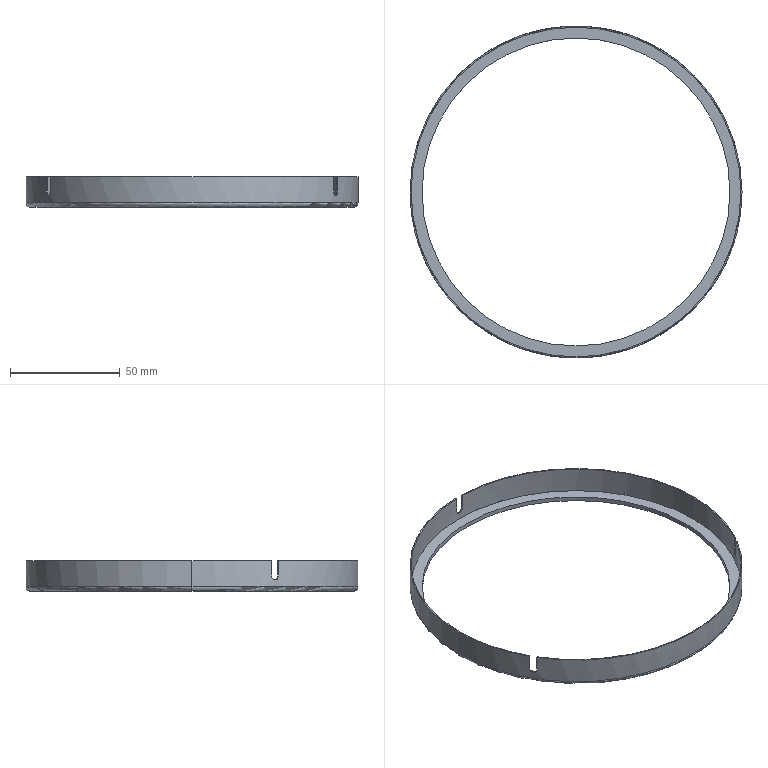Part | SolidWorks | features ICE 3, CirPattern 1, Extrusion 1, Fillet 1 | 1 solid | 22 faces | box 151 x 151 x 14 mm | volume 7416 mm3 | plane 11 | cylinder 9 | torus 2 | commonest cylinder face diameters 3.5 x3 140 x2 150 x2 151 x2
STEP:
#1=CARTESIAN_POINT('',(-73.5,0.,0.));
#2=VERTEX_POINT('',#1);
#3=CARTESIAN_POINT('',(73.5,0.,0.));
#4=VERTEX_POINT('',#3);
#5=CARTESIAN_POINT('',(0.,0.,0.));
#6=DIRECTION('',(0.,0.,-1.));
#7=DIRECTION('',(1.,0.,0.));
#8=AXIS2_PLACEMENT_3D('',#5,#6,#7);
#9=CIRCLE('',#8,73.5);
#10=EDGE_CURVE('',#2,#4,#9,.T.);
#11=ORIENTED_EDGE('',*,*,#10,.F.);
#12=CARTESIAN_POINT('',(-75.5,0.,2.));
#13=VERTEX_POINT('',#12);
#14=CARTESIAN_POINT('',(-73.5,0.,2.));
#15=DIRECTION('',(0.,1.,0.));
#16=DIRECTION('',(-1.,0.,0.));
#17=AXIS2_PLACEMENT_3D('',#14,#15,#16);
#18=CIRCLE('',#17,2.);
#19=EDGE_CURVE('',#2,#13,#18,.T.);
#20=ORIENTED_EDGE('',*,*,#19,.T.);
#21=CARTESIAN_POINT('',(75.5,0.,2.));
#22=VERTEX_POINT('',#21);
#23=CARTESIAN_POINT('',(0.,0.,2.));
#24=DIRECTION('',(0.,0.,1.));
#25=DIRECTION('',(1.,0.,0.));
#26=AXIS2_PLACEMENT_3D('',#23,#24,#25);
#27=CIRCLE('',#26,75.5);
#28=EDGE_CURVE('',#22,#13,#27,.T.);
#29=ORIENTED_EDGE('',*,*,#28,.F.);
#30=CARTESIAN_POINT('',(73.5,0.,2.));
#31=DIRECTION('',(0.,-1.,0.));
#32=DIRECTION('',(0.,0.,-1.));
#33=AXIS2_PLACEMENT_3D('',#30,#31,#32);
#34=CIRCLE('',#33,2.);
#35=EDGE_CURVE('',#4,#22,#34,.T.);
#36=ORIENTED_EDGE('',*,*,#35,.F.);
#37=EDGE_LOOP('',(#11,#20,#29,#36));
#38=FACE_OUTER_BOUND('',#37,.T.);
#39=CARTESIAN_POINT('',(0.,0.,2.));
#40=DIRECTION('',(0.,0.,1.));
#41=DIRECTION('',(1.,0.,0.));
#42=AXIS2_PLACEMENT_3D('',#39,#40,#41);
#43=TOROIDAL_SURFACE('',#42,73.5,2.);
#44=ADVANCED_FACE('',(#38),#43,.T.);
#45=CARTESIAN_POINT('',(70.,0.,2.));
#46=VERTEX_POINT('',#45);
#47=CARTESIAN_POINT('',(-70.,0.,2.));
#48=VERTEX_POINT('',#47);
#49=CARTESIAN_POINT('',(0.,0.,2.));
#50=DIRECTION('',(0.,0.,-1.));
#51=DIRECTION('',(1.,0.,0.));
#52=AXIS2_PLACEMENT_3D('',#49,#50,#51);
#53=CIRCLE('',#52,70.);
#54=EDGE_CURVE('',#46,#48,#53,.T.);
#55=ORIENTED_EDGE('',*,*,#54,.F.);
#56=CARTESIAN_POINT('',(70.,0.,0.));
#57=VERTEX_POINT('',#56);
#58=CARTESIAN_POINT('',(70.,0.,14.001));
#59=DIRECTION('',(0.,0.,-1.));
#60=VECTOR('',#59,1000.);
#61=LINE('',#58,#60);
#62=EDGE_CURVE('',#46,#57,#61,.T.);
#63=ORIENTED_EDGE('',*,*,#62,.T.);
#64=CARTESIAN_POINT('',(-70.,0.,0.));
#65=VERTEX_POINT('',#64);
#66=CARTESIAN_POINT('',(0.,0.,0.));
#67=DIRECTION('',(0.,0.,-1.));
#68=DIRECTION('',(-1.,0.,0.));
#69=AXIS2_PLACEMENT_3D('',#66,#67,#68);
#70=CIRCLE('',#69,70.);
#71=EDGE_CURVE('',#57,#65,#70,.T.);
#72=ORIENTED_EDGE('',*,*,#71,.T.);
#73=CARTESIAN_POINT('',(-70.,0.,14.001));
#74=DIRECTION('',(0.,0.,-1.));
#75=VECTOR('',#74,1000.);
#76=LINE('',#73,#75);
#77=EDGE_CURVE('',#48,#65,#76,.T.);
#78=ORIENTED_EDGE('',*,*,#77,.F.);
#79=EDGE_LOOP('',(#55,#63,#72,#78));
#80=FACE_OUTER_BOUND('',#79,.T.);
#81=CARTESIAN_POINT('',(0.,0.,14.001));
#82=DIRECTION('',(0.,0.,-1.));
#83=DIRECTION('',(-1.,0.,0.));
#84=AXIS2_PLACEMENT_3D('',#81,#82,#83);
#85=CYLINDRICAL_SURFACE('',#84,70.);
#86=ADVANCED_FACE('',(#80),#85,.F.);
#87=CARTESIAN_POINT('',(65.809,-35.974,14.));
#88=VERTEX_POINT('',#87);
#89=CARTESIAN_POINT('',(75.,0.,14.));
#90=VERTEX_POINT('',#89);
#91=CARTESIAN_POINT('',(0.,0.,14.));
#92=DIRECTION('',(0.,0.,1.));
#93=DIRECTION('',(1.,0.,0.));
#94=AXIS2_PLACEMENT_3D('',#91,#92,#93);
#95=CIRCLE('',#94,75.);
#96=EDGE_CURVE('',#88,#90,#95,.T.);
#97=ORIENTED_EDGE('',*,*,#96,.T.);
#98=CARTESIAN_POINT('',(75.,0.,2.));
#99=VERTEX_POINT('',#98);
#100=CARTESIAN_POINT('',(75.,0.,14.));
#101=DIRECTION('',(0.,0.,-1.));
#102=VECTOR('',#101,1000.);
#103=LINE('',#100,#102);
#104=EDGE_CURVE('',#90,#99,#103,.T.);
#105=ORIENTED_EDGE('',*,*,#104,.T.);
#106=CARTESIAN_POINT('',(-75.,0.,2.));
#107=VERTEX_POINT('',#106);
#108=CARTESIAN_POINT('',(0.,0.,2.));
#109=DIRECTION('',(0.,0.,1.));
#110=DIRECTION('',(1.,0.,0.));
#111=AXIS2_PLACEMENT_3D('',#108,#109,#110);
#112=CIRCLE('',#111,75.);
#113=EDGE_CURVE('',#107,#99,#112,.T.);
#114=ORIENTED_EDGE('',*,*,#113,.F.);
#115=CARTESIAN_POINT('',(-75.,0.,14.));
#116=VERTEX_POINT('',#115);
#117=CARTESIAN_POINT('',(-75.,0.,14.));
#118=DIRECTION('',(0.,0.,-1.));
#119=VECTOR('',#118,1000.);
#120=LINE('',#117,#119);
#121=EDGE_CURVE('',#116,#107,#120,.T.);
#122=ORIENTED_EDGE('',*,*,#121,.F.);
#123=CARTESIAN_POINT('',(-65.809,-35.974,14.));
#124=VERTEX_POINT('',#123);
#125=CARTESIAN_POINT('',(0.,0.,14.));
#126=DIRECTION('',(0.,0.,1.));
#127=DIRECTION('',(1.,0.,0.));
#128=AXIS2_PLACEMENT_3D('',#125,#126,#127);
#129=CIRCLE('',#128,75.);
#130=EDGE_CURVE('',#116,#124,#129,.T.);
#131=ORIENTED_EDGE('',*,*,#130,.T.);
#132=CARTESIAN_POINT('',(-65.809,-35.974,7.));
#133=VERTEX_POINT('',#132);
#134=CARTESIAN_POINT('',(-65.809,-35.974,14.));
#135=DIRECTION('',(0.,0.,-1.));
#136=VECTOR('',#135,1000.);
#137=LINE('',#134,#136);
#138=EDGE_CURVE('',#124,#133,#137,.T.);
#139=ORIENTED_EDGE('',*,*,#138,.T.);
#140=CARTESIAN_POINT('',(-64.059,-39.005,7.));
#141=VERTEX_POINT('',#140);
#142=CARTESIAN_POINT('',(-64.059,-39.005,7.));
#143=CARTESIAN_POINT('',(-64.059,-39.005,6.884));
#144=CARTESIAN_POINT('',(-64.065,-38.996,6.771));
#145=CARTESIAN_POINT('',(-64.088,-38.958,6.547));
#146=CARTESIAN_POINT('',(-64.106,-38.929,6.436));
#147=CARTESIAN_POINT('',(-64.151,-38.854,6.224));
#148=CARTESIAN_POINT('',(-64.179,-38.808,6.124));
#149=CARTESIAN_POINT('',(-64.245,-38.699,5.933));
#150=CARTESIAN_POINT('',(-64.283,-38.636,5.843));
#151=CARTESIAN_POINT('',(-64.407,-38.428,5.601));
#152=CARTESIAN_POINT('',(-64.507,-38.26,5.471));
#153=CARTESIAN_POINT('',(-64.721,-37.898,5.296));
#154=CARTESIAN_POINT('',(-64.837,-37.699,5.25));
#155=CARTESIAN_POINT('',(-65.008,-37.402,5.25));
#156=CARTESIAN_POINT('',(-65.066,-37.302,5.261));
#157=CARTESIAN_POINT('',(-65.177,-37.107,5.306));
#158=CARTESIAN_POINT('',(-65.231,-37.012,5.339));
#159=CARTESIAN_POINT('',(-65.336,-36.828,5.426));
#160=CARTESIAN_POINT('',(-65.386,-36.738,5.481));
#161=CARTESIAN_POINT('',(-65.479,-36.573,5.608));
#162=CARTESIAN_POINT('',(-65.522,-36.495,5.68));
#163=CARTESIAN_POINT('',(-65.601,-36.353,5.843));
#164=CARTESIAN_POINT('',(-65.636,-36.289,5.932));
#165=CARTESIAN_POINT('',(-65.697,-36.178,6.121));
#166=CARTESIAN_POINT('',(-65.724,-36.13,6.223));
#167=CARTESIAN_POINT('',(-65.787,-36.014,6.541));
#168=CARTESIAN_POINT('',(-65.809,-35.974,6.769));
#169=CARTESIAN_POINT('',(-65.809,-35.974,7.));
#170=B_SPLINE_CURVE_WITH_KNOTS('',3,(#142,#143,#144,#145,#146,#147,#148,#149,#150,#151,#152,#153,#154,#155,#156,#157,#158,#159,#160,#161,#162,#163,#164,#165,#166,#167,#168,#169),.UNSPECIFIED.,.F.,.F.,(4,2,2,2,2,2,2,2,2,2,2,2,2,4),(0.,0.0003419,0.0006838,0.001026,0.001368,0.002051,0.002735,0.003077,0.003419,0.003761,0.004103,0.004445,0.004787,0.00547),.UNSPECIFIED.);
#171=EDGE_CURVE('',#141,#133,#170,.T.);
#172=ORIENTED_EDGE('',*,*,#171,.F.);
#173=CARTESIAN_POINT('',(-64.059,-39.005,14.));
#174=VERTEX_POINT('',#173);
#175=CARTESIAN_POINT('',(-64.059,-39.005,14.));
#176=DIRECTION('',(0.,0.,-1.));
#177=VECTOR('',#176,1000.);
#178=LINE('',#175,#177);
#179=EDGE_CURVE('',#174,#141,#178,.T.);
#180=ORIENTED_EDGE('',*,*,#179,.F.);
#181=CARTESIAN_POINT('',(64.059,-39.005,14.));
#182=VERTEX_POINT('',#181);
#183=CARTESIAN_POINT('',(0.,0.,14.));
#184=DIRECTION('',(0.,0.,1.));
#185=DIRECTION('',(1.,0.,0.));
#186=AXIS2_PLACEMENT_3D('',#183,#184,#185);
#187=CIRCLE('',#186,75.);
#188=EDGE_CURVE('',#174,#182,#187,.T.);
#189=ORIENTED_EDGE('',*,*,#188,.T.);
#190=CARTESIAN_POINT('',(64.059,-39.005,7.));
#191=VERTEX_POINT('',#190);
#192=CARTESIAN_POINT('',(64.059,-39.005,14.));
#193=DIRECTION('',(0.,0.,-1.));
#194=VECTOR('',#193,1000.);
#195=LINE('',#192,#194);
#196=EDGE_CURVE('',#182,#191,#195,.T.);
#197=ORIENTED_EDGE('',*,*,#196,.T.);
#198=CARTESIAN_POINT('',(65.809,-35.974,7.));
#199=VERTEX_POINT('',#198);
#200=CARTESIAN_POINT('',(65.809,-35.974,7.));
#201=CARTESIAN_POINT('',(65.809,-35.974,6.884));
#202=CARTESIAN_POINT('',(65.804,-35.984,6.771));
#203=CARTESIAN_POINT('',(65.782,-36.023,6.547));
#204=CARTESIAN_POINT('',(65.766,-36.053,6.436));
#205=CARTESIAN_POINT('',(65.724,-36.13,6.224));
#206=CARTESIAN_POINT('',(65.698,-36.177,6.124));
#207=CARTESIAN_POINT('',(65.637,-36.288,5.933));
#208=CARTESIAN_POINT('',(65.601,-36.353,5.843));
#209=CARTESIAN_POINT('',(65.483,-36.564,5.601));
#210=CARTESIAN_POINT('',(65.388,-36.735,5.471));
#211=CARTESIAN_POINT('',(65.181,-37.101,5.296));
#212=CARTESIAN_POINT('',(65.067,-37.301,5.25));
#213=CARTESIAN_POINT('',(64.895,-37.598,5.25));
#214=CARTESIAN_POINT('',(64.837,-37.698,5.261));
#215=CARTESIAN_POINT('',(64.724,-37.892,5.306));
#216=CARTESIAN_POINT('',(64.669,-37.986,5.339));
#217=CARTESIAN_POINT('',(64.561,-38.169,5.426));
#218=CARTESIAN_POINT('',(64.509,-38.257,5.481));
#219=CARTESIAN_POINT('',(64.412,-38.42,5.608));
#220=CARTESIAN_POINT('',(64.367,-38.496,5.68));
#221=CARTESIAN_POINT('',(64.283,-38.636,5.843));
#222=CARTESIAN_POINT('',(64.245,-38.698,5.932));
#223=CARTESIAN_POINT('',(64.18,-38.807,6.121));
#224=CARTESIAN_POINT('',(64.151,-38.854,6.223));
#225=CARTESIAN_POINT('',(64.083,-38.966,6.541));
#226=CARTESIAN_POINT('',(64.059,-39.005,6.769));
#227=CARTESIAN_POINT('',(64.059,-39.005,7.));
#228=B_SPLINE_CURVE_WITH_KNOTS('',3,(#200,#201,#202,#203,#204,#205,#206,#207,#208,#209,#210,#211,#212,#213,#214,#215,#216,#217,#218,#219,#220,#221,#222,#223,#224,#225,#226,#227),.UNSPECIFIED.,.F.,.F.,(4,2,2,2,2,2,2,2,2,2,2,2,2,4),(0.,0.0003419,0.0006838,0.001026,0.001368,0.002051,0.002735,0.003077,0.003419,0.003761,0.004103,0.004445,0.004787,0.00547),.UNSPECIFIED.);
#229=EDGE_CURVE('',#199,#191,#228,.T.);
#230=ORIENTED_EDGE('',*,*,#229,.F.);
#231=CARTESIAN_POINT('',(65.809,-35.974,14.));
#232=DIRECTION('',(0.,0.,-1.));
#233=VECTOR('',#232,1000.);
#234=LINE('',#231,#233);
#235=EDGE_CURVE('',#88,#199,#234,.T.);
#236=ORIENTED_EDGE('',*,*,#235,.F.);
#237=EDGE_LOOP('',(#97,#105,#114,#122,#131,#139,#172,#180,#189,#197,#230,#236));
#238=FACE_OUTER_BOUND('',#237,.T.);
#239=CARTESIAN_POINT('',(0.,0.,14.));
#240=DIRECTION('',(0.,0.,-1.));
#241=DIRECTION('',(-1.,0.,0.));
#242=AXIS2_PLACEMENT_3D('',#239,#240,#241);
#243=CYLINDRICAL_SURFACE('',#242,75.);
#244=ADVANCED_FACE('',(#238),#243,.F.);
#245=CARTESIAN_POINT('',(75.5,0.,14.));
#246=VERTEX_POINT('',#245);
#247=CARTESIAN_POINT('',(1.75,75.48,14.));
#248=VERTEX_POINT('',#247);
#249=CARTESIAN_POINT('',(0.,0.,14.));
#250=DIRECTION('',(0.,0.,1.));
#251=DIRECTION('',(1.,0.,0.));
#252=AXIS2_PLACEMENT_3D('',#249,#250,#251);
#253=CIRCLE('',#252,75.5);
#254=EDGE_CURVE('',#246,#248,#253,.T.);
#255=ORIENTED_EDGE('',*,*,#254,.F.);
#256=CARTESIAN_POINT('',(75.5,0.,14.));
#257=DIRECTION('',(0.,0.,-1.));
#258=VECTOR('',#257,1000.);
#259=LINE('',#256,#258);
#260=EDGE_CURVE('',#246,#22,#259,.T.);
#261=ORIENTED_EDGE('',*,*,#260,.T.);
#262=ORIENTED_EDGE('',*,*,#28,.T.);
#263=CARTESIAN_POINT('',(-75.5,0.,14.));
#264=VERTEX_POINT('',#263);
#265=CARTESIAN_POINT('',(-75.5,0.,14.));
#266=DIRECTION('',(0.,0.,-1.));
#267=VECTOR('',#266,1000.);
#268=LINE('',#265,#267);
#269=EDGE_CURVE('',#264,#13,#268,.T.);
#270=ORIENTED_EDGE('',*,*,#269,.F.);
#271=CARTESIAN_POINT('',(-1.75,75.48,14.));
#272=VERTEX_POINT('',#271);
#273=CARTESIAN_POINT('',(0.,0.,14.));
#274=DIRECTION('',(0.,0.,1.));
#275=DIRECTION('',(1.,0.,0.));
#276=AXIS2_PLACEMENT_3D('',#273,#274,#275);
#277=CIRCLE('',#276,75.5);
#278=EDGE_CURVE('',#272,#264,#277,.T.);
#279=ORIENTED_EDGE('',*,*,#278,.F.);
#280=CARTESIAN_POINT('',(-1.75,75.48,7.));
#281=VERTEX_POINT('',#280);
#282=CARTESIAN_POINT('',(-1.75,75.48,14.));
#283=DIRECTION('',(0.,0.,-1.));
#284=VECTOR('',#283,1000.);
#285=LINE('',#282,#284);
#286=EDGE_CURVE('',#272,#281,#285,.T.);
#287=ORIENTED_EDGE('',*,*,#286,.T.);
#288=CARTESIAN_POINT('',(1.75,75.48,7.));
#289=VERTEX_POINT('',#288);
#290=CARTESIAN_POINT('',(-1.75,75.48,7.));
#291=CARTESIAN_POINT('',(-1.75,75.48,6.884));
#292=CARTESIAN_POINT('',(-1.739,75.48,6.771));
#293=CARTESIAN_POINT('',(-1.694,75.481,6.547));
#294=CARTESIAN_POINT('',(-1.661,75.482,6.436));
#295=CARTESIAN_POINT('',(-1.573,75.484,6.224));
#296=CARTESIAN_POINT('',(-1.519,75.485,6.124));
#297=CARTESIAN_POINT('',(-1.392,75.487,5.933));
#298=CARTESIAN_POINT('',(-1.318,75.489,5.843));
#299=CARTESIAN_POINT('',(-1.076,75.493,5.601));
#300=CARTESIAN_POINT('',(-0.8808,75.495,5.471));
#301=CARTESIAN_POINT('',(-0.4597,75.499,5.296));
#302=CARTESIAN_POINT('',(-0.2294,75.5,5.25));
#303=CARTESIAN_POINT('',(0.1129,75.5,5.25));
#304=CARTESIAN_POINT('',(0.2288,75.5,5.261));
#305=CARTESIAN_POINT('',(0.4533,75.499,5.306));
#306=CARTESIAN_POINT('',(0.5624,75.498,5.339));
#307=CARTESIAN_POINT('',(0.7742,75.496,5.426));
#308=CARTESIAN_POINT('',(0.8767,75.495,5.481));
#309=CARTESIAN_POINT('',(1.066,75.493,5.608));
#310=CARTESIAN_POINT('',(1.155,75.491,5.68));
#311=CARTESIAN_POINT('',(1.318,75.489,5.843));
#312=CARTESIAN_POINT('',(1.391,75.487,5.932));
#313=CARTESIAN_POINT('',(1.518,75.485,6.121));
#314=CARTESIAN_POINT('',(1.572,75.484,6.223));
#315=CARTESIAN_POINT('',(1.704,75.481,6.541));
#316=CARTESIAN_POINT('',(1.75,75.48,6.769));
#317=CARTESIAN_POINT('',(1.75,75.48,7.));
#318=B_SPLINE_CURVE_WITH_KNOTS('',3,(#290,#291,#292,#293,#294,#295,#296,#297,#298,#299,#300,#301,#302,#303,#304,#305,#306,#307,#308,#309,#310,#311,#312,#313,#314,#315,#316,#317),.UNSPECIFIED.,.F.,.F.,(4,2,2,2,2,2,2,2,2,2,2,2,2,4),(0.,0.0003419,0.0006838,0.001026,0.001368,0.002051,0.002735,0.003077,0.003419,0.003761,0.004103,0.004445,0.004787,0.00547),.UNSPECIFIED.);
#319=EDGE_CURVE('',#281,#289,#318,.T.);
#320=ORIENTED_EDGE('',*,*,#319,.T.);
#321=CARTESIAN_POINT('',(1.75,75.48,14.));
#322=DIRECTION('',(0.,0.,-1.));
#323=VECTOR('',#322,1000.);
#324=LINE('',#321,#323);
#325=EDGE_CURVE('',#248,#289,#324,.T.);
#326=ORIENTED_EDGE('',*,*,#325,.F.);
#327=EDGE_LOOP('',(#255,#261,#262,#270,#279,#287,#320,#326));
#328=FACE_OUTER_BOUND('',#327,.T.);
#329=CARTESIAN_POINT('',(0.,0.,14.));
#330=DIRECTION('',(0.,0.,-1.));
#331=DIRECTION('',(-1.,0.,0.));
#332=AXIS2_PLACEMENT_3D('',#329,#330,#331);
#333=CYLINDRICAL_SURFACE('',#332,75.5);
#334=ADVANCED_FACE('',(#328),#333,.T.);
#335=ORIENTED_EDGE('',*,*,#96,.F.);
#336=CARTESIAN_POINT('',(66.242,-36.224,14.));
#337=VERTEX_POINT('',#336);
#338=CARTESIAN_POINT('',(-88.444,53.084,14.));
#339=DIRECTION('',(0.866,-0.5,0.));
#340=VECTOR('',#339,1000.);
#341=LINE('',#338,#340);
#342=EDGE_CURVE('',#88,#337,#341,.T.);
#343=ORIENTED_EDGE('',*,*,#342,.T.);
#344=CARTESIAN_POINT('',(0.,0.,14.));
#345=DIRECTION('',(0.,0.,1.));
#346=DIRECTION('',(1.,0.,0.));
#347=AXIS2_PLACEMENT_3D('',#344,#345,#346);
#348=CIRCLE('',#347,75.5);
#349=EDGE_CURVE('',#337,#246,#348,.T.);
#350=ORIENTED_EDGE('',*,*,#349,.T.);
#351=ORIENTED_EDGE('',*,*,#254,.T.);
#352=CARTESIAN_POINT('',(1.75,74.98,14.));
#353=VERTEX_POINT('',#352);
#354=CARTESIAN_POINT('',(1.75,-75.501,14.));
#355=DIRECTION('',(0.,1.,0.));
#356=VECTOR('',#355,1000.);
#357=LINE('',#354,#356);
#358=EDGE_CURVE('',#353,#248,#357,.T.);
#359=ORIENTED_EDGE('',*,*,#358,.F.);
#360=CARTESIAN_POINT('',(0.,0.,14.));
#361=DIRECTION('',(0.,0.,1.));
#362=DIRECTION('',(1.,0.,0.));
#363=AXIS2_PLACEMENT_3D('',#360,#361,#362);
#364=CIRCLE('',#363,75.);
#365=EDGE_CURVE('',#90,#353,#364,.T.);
#366=ORIENTED_EDGE('',*,*,#365,.F.);
#367=EDGE_LOOP('',(#335,#343,#350,#351,#359,#366));
#368=FACE_OUTER_BOUND('',#367,.T.);
#369=CARTESIAN_POINT('',(0.,0.,14.));
#370=DIRECTION('',(0.,0.,1.));
#371=DIRECTION('',(1.,0.,0.));
#372=AXIS2_PLACEMENT_3D('',#369,#370,#371);
#373=PLANE('',#372);
#374=ADVANCED_FACE('',(#368),#373,.T.);
#375=CARTESIAN_POINT('',(64.492,-39.255,14.));
#376=VERTEX_POINT('',#375);
#377=CARTESIAN_POINT('',(-90.194,50.053,14.));
#378=DIRECTION('',(0.866,-0.5,0.));
#379=VECTOR('',#378,1000.);
#380=LINE('',#377,#379);
#381=EDGE_CURVE('',#182,#376,#380,.T.);
#382=ORIENTED_EDGE('',*,*,#381,.F.);
#383=ORIENTED_EDGE('',*,*,#188,.F.);
#384=CARTESIAN_POINT('',(-64.492,-39.255,14.));
#385=VERTEX_POINT('',#384);
#386=CARTESIAN_POINT('',(90.194,50.053,14.));
#387=DIRECTION('',(-0.866,-0.5,0.));
#388=VECTOR('',#387,1000.);
#389=LINE('',#386,#388);
#390=EDGE_CURVE('',#174,#385,#389,.T.);
#391=ORIENTED_EDGE('',*,*,#390,.T.);
#392=CARTESIAN_POINT('',(0.,0.,14.));
#393=DIRECTION('',(0.,0.,1.));
#394=DIRECTION('',(1.,0.,0.));
#395=AXIS2_PLACEMENT_3D('',#392,#393,#394);
#396=CIRCLE('',#395,75.5);
#397=EDGE_CURVE('',#385,#376,#396,.T.);
#398=ORIENTED_EDGE('',*,*,#397,.T.);
#399=EDGE_LOOP('',(#382,#383,#391,#398));
#400=FACE_OUTER_BOUND('',#399,.T.);
#401=CARTESIAN_POINT('',(0.,0.,14.));
#402=DIRECTION('',(0.,0.,1.));
#403=DIRECTION('',(1.,0.,0.));
#404=AXIS2_PLACEMENT_3D('',#401,#402,#403);
#405=PLANE('',#404);
#406=ADVANCED_FACE('',(#400),#405,.T.);
#407=ORIENTED_EDGE('',*,*,#260,.F.);
#408=ORIENTED_EDGE('',*,*,#349,.F.);
#409=CARTESIAN_POINT('',(66.242,-36.224,7.));
#410=VERTEX_POINT('',#409);
#411=CARTESIAN_POINT('',(66.242,-36.224,14.));
#412=DIRECTION('',(0.,0.,-1.));
#413=VECTOR('',#412,1000.);
#414=LINE('',#411,#413);
#415=EDGE_CURVE('',#337,#410,#414,.T.);
#416=ORIENTED_EDGE('',*,*,#415,.T.);
#417=CARTESIAN_POINT('',(64.492,-39.255,7.));
#418=VERTEX_POINT('',#417);
#419=CARTESIAN_POINT('',(66.242,-36.224,7.));
#420=CARTESIAN_POINT('',(66.242,-36.224,6.884));
#421=CARTESIAN_POINT('',(66.237,-36.234,6.771));
#422=CARTESIAN_POINT('',(66.216,-36.273,6.547));
#423=CARTESIAN_POINT('',(66.199,-36.303,6.436));
#424=CARTESIAN_POINT('',(66.157,-36.38,6.224));
#425=CARTESIAN_POINT('',(66.131,-36.427,6.124));
#426=CARTESIAN_POINT('',(66.07,-36.538,5.933));
#427=CARTESIAN_POINT('',(66.034,-36.603,5.843));
#428=CARTESIAN_POINT('',(65.916,-36.814,5.601));
#429=CARTESIAN_POINT('',(65.821,-36.985,5.471));
#430=CARTESIAN_POINT('',(65.614,-37.351,5.296));
#431=CARTESIAN_POINT('',(65.5,-37.551,5.25));
#432=CARTESIAN_POINT('',(65.328,-37.848,5.25));
#433=CARTESIAN_POINT('',(65.27,-37.948,5.261));
#434=CARTESIAN_POINT('',(65.157,-38.142,5.306));
#435=CARTESIAN_POINT('',(65.102,-38.236,5.339));
#436=CARTESIAN_POINT('',(64.994,-38.419,5.426));
#437=CARTESIAN_POINT('',(64.942,-38.507,5.481));
#438=CARTESIAN_POINT('',(64.845,-38.67,5.608));
#439=CARTESIAN_POINT('',(64.8,-38.746,5.68));
#440=CARTESIAN_POINT('',(64.716,-38.886,5.843));
#441=CARTESIAN_POINT('',(64.678,-38.948,5.932));
#442=CARTESIAN_POINT('',(64.613,-39.057,6.121));
#443=CARTESIAN_POINT('',(64.585,-39.104,6.223));
#444=CARTESIAN_POINT('',(64.516,-39.216,6.541));
#445=CARTESIAN_POINT('',(64.492,-39.255,6.769));
#446=CARTESIAN_POINT('',(64.492,-39.255,7.));
#447=B_SPLINE_CURVE_WITH_KNOTS('',3,(#419,#420,#421,#422,#423,#424,#425,#426,#427,#428,#429,#430,#431,#432,#433,#434,#435,#436,#437,#438,#439,#440,#441,#442,#443,#444,#445,#446),.UNSPECIFIED.,.F.,.F.,(4,2,2,2,2,2,2,2,2,2,2,2,2,4),(0.,0.0003419,0.0006838,0.001026,0.001368,0.002051,0.002735,0.003077,0.003419,0.003761,0.004103,0.004445,0.004787,0.00547),.UNSPECIFIED.);
#448=EDGE_CURVE('',#410,#418,#447,.T.);
#449=ORIENTED_EDGE('',*,*,#448,.T.);
#450=CARTESIAN_POINT('',(64.492,-39.255,14.));
#451=DIRECTION('',(0.,0.,-1.));
#452=VECTOR('',#451,1000.);
#453=LINE('',#450,#452);
#454=EDGE_CURVE('',#376,#418,#453,.T.);
#455=ORIENTED_EDGE('',*,*,#454,.F.);
#456=ORIENTED_EDGE('',*,*,#397,.F.);
#457=CARTESIAN_POINT('',(-64.492,-39.255,7.));
#458=VERTEX_POINT('',#457);
#459=CARTESIAN_POINT('',(-64.492,-39.255,14.));
#460=DIRECTION('',(0.,0.,-1.));
#461=VECTOR('',#460,1000.);
#462=LINE('',#459,#461);
#463=EDGE_CURVE('',#385,#458,#462,.T.);
#464=ORIENTED_EDGE('',*,*,#463,.T.);
#465=CARTESIAN_POINT('',(-66.242,-36.224,7.));
#466=VERTEX_POINT('',#465);
#467=CARTESIAN_POINT('',(-64.492,-39.255,7.));
#468=CARTESIAN_POINT('',(-64.492,-39.255,6.884));
#469=CARTESIAN_POINT('',(-64.498,-39.246,6.771));
#470=CARTESIAN_POINT('',(-64.521,-39.208,6.547));
#471=CARTESIAN_POINT('',(-64.539,-39.179,6.436));
#472=CARTESIAN_POINT('',(-64.584,-39.104,6.224));
#473=CARTESIAN_POINT('',(-64.612,-39.058,6.124));
#474=CARTESIAN_POINT('',(-64.678,-38.949,5.933));
#475=CARTESIAN_POINT('',(-64.716,-38.886,5.843));
#476=CARTESIAN_POINT('',(-64.84,-38.678,5.601));
#477=CARTESIAN_POINT('',(-64.94,-38.51,5.471));
#478=CARTESIAN_POINT('',(-65.154,-38.148,5.296));
#479=CARTESIAN_POINT('',(-65.27,-37.949,5.25));
#480=CARTESIAN_POINT('',(-65.441,-37.652,5.25));
#481=CARTESIAN_POINT('',(-65.499,-37.552,5.261));
#482=CARTESIAN_POINT('',(-65.61,-37.357,5.306));
#483=CARTESIAN_POINT('',(-65.664,-37.262,5.339));
#484=CARTESIAN_POINT('',(-65.769,-37.078,5.426));
#485=CARTESIAN_POINT('',(-65.819,-36.988,5.481));
#486=CARTESIAN_POINT('',(-65.912,-36.823,5.608));
#487=CARTESIAN_POINT('',(-65.955,-36.746,5.68));
#488=CARTESIAN_POINT('',(-66.034,-36.603,5.843));
#489=CARTESIAN_POINT('',(-66.069,-36.539,5.932));
#490=CARTESIAN_POINT('',(-66.131,-36.428,6.121));
#491=CARTESIAN_POINT('',(-66.157,-36.38,6.223));
#492=CARTESIAN_POINT('',(-66.22,-36.264,6.541));
#493=CARTESIAN_POINT('',(-66.242,-36.224,6.769));
#494=CARTESIAN_POINT('',(-66.242,-36.224,7.));
#495=B_SPLINE_CURVE_WITH_KNOTS('',3,(#467,#468,#469,#470,#471,#472,#473,#474,#475,#476,#477,#478,#479,#480,#481,#482,#483,#484,#485,#486,#487,#488,#489,#490,#491,#492,#493,#494),.UNSPECIFIED.,.F.,.F.,(4,2,2,2,2,2,2,2,2,2,2,2,2,4),(0.,0.0003419,0.0006838,0.001026,0.001368,0.002051,0.002735,0.003077,0.003419,0.003761,0.004103,0.004445,0.004787,0.00547),.UNSPECIFIED.);
#496=EDGE_CURVE('',#458,#466,#495,.T.);
#497=ORIENTED_EDGE('',*,*,#496,.T.);
#498=CARTESIAN_POINT('',(-66.242,-36.224,14.));
#499=VERTEX_POINT('',#498);
#500=CARTESIAN_POINT('',(-66.242,-36.224,14.));
#501=DIRECTION('',(0.,0.,-1.));
#502=VECTOR('',#501,1000.);
#503=LINE('',#500,#502);
#504=EDGE_CURVE('',#499,#466,#503,.T.);
#505=ORIENTED_EDGE('',*,*,#504,.F.);
#506=CARTESIAN_POINT('',(0.,0.,14.));
#507=DIRECTION('',(0.,0.,1.));
#508=DIRECTION('',(1.,0.,0.));
#509=AXIS2_PLACEMENT_3D('',#506,#507,#508);
#510=CIRCLE('',#509,75.5);
#511=EDGE_CURVE('',#264,#499,#510,.T.);
#512=ORIENTED_EDGE('',*,*,#511,.F.);
#513=ORIENTED_EDGE('',*,*,#269,.T.);
#514=CARTESIAN_POINT('',(0.,0.,2.));
#515=DIRECTION('',(0.,0.,1.));
#516=DIRECTION('',(1.,0.,0.));
#517=AXIS2_PLACEMENT_3D('',#514,#515,#516);
#518=CIRCLE('',#517,75.5);
#519=EDGE_CURVE('',#13,#22,#518,.T.);
#520=ORIENTED_EDGE('',*,*,#519,.T.);
#521=EDGE_LOOP('',(#407,#408,#416,#449,#455,#456,#464,#497,#505,#512,#513,#520));
#522=FACE_OUTER_BOUND('',#521,.T.);
#523=CARTESIAN_POINT('',(0.,0.,14.));
#524=DIRECTION('',(0.,0.,-1.));
#525=DIRECTION('',(-1.,0.,0.));
#526=AXIS2_PLACEMENT_3D('',#523,#524,#525);
#527=CYLINDRICAL_SURFACE('',#526,75.5);
#528=ADVANCED_FACE('',(#522),#527,.T.);
#529=ORIENTED_EDGE('',*,*,#104,.F.);
#530=ORIENTED_EDGE('',*,*,#365,.T.);
#531=CARTESIAN_POINT('',(1.75,74.98,7.));
#532=VERTEX_POINT('',#531);
#533=CARTESIAN_POINT('',(1.75,74.98,14.));
#534=DIRECTION('',(0.,0.,-1.));
#535=VECTOR('',#534,1000.);
#536=LINE('',#533,#535);
#537=EDGE_CURVE('',#353,#532,#536,.T.);
#538=ORIENTED_EDGE('',*,*,#537,.T.);
#539=CARTESIAN_POINT('',(-1.75,74.98,7.));
#540=VERTEX_POINT('',#539);
#541=CARTESIAN_POINT('',(-1.75,74.98,7.));
#542=CARTESIAN_POINT('',(-1.75,74.98,6.884));
#543=CARTESIAN_POINT('',(-1.739,74.98,6.771));
#544=CARTESIAN_POINT('',(-1.694,74.981,6.547));
#545=CARTESIAN_POINT('',(-1.661,74.982,6.436));
#546=CARTESIAN_POINT('',(-1.573,74.984,6.224));
#547=CARTESIAN_POINT('',(-1.519,74.985,6.124));
#548=CARTESIAN_POINT('',(-1.392,74.987,5.933));
#549=CARTESIAN_POINT('',(-1.318,74.988,5.843));
#550=CARTESIAN_POINT('',(-1.076,74.992,5.601));
#551=CARTESIAN_POINT('',(-0.8808,74.995,5.471));
#552=CARTESIAN_POINT('',(-0.4597,74.999,5.296));
#553=CARTESIAN_POINT('',(-0.2294,75.,5.25));
#554=CARTESIAN_POINT('',(0.1129,75.,5.25));
#555=CARTESIAN_POINT('',(0.2288,75.,5.261));
#556=CARTESIAN_POINT('',(0.4533,74.999,5.306));
#557=CARTESIAN_POINT('',(0.5624,74.998,5.339));
#558=CARTESIAN_POINT('',(0.7742,74.996,5.426));
#559=CARTESIAN_POINT('',(0.8767,74.995,5.481));
#560=CARTESIAN_POINT('',(1.066,74.992,5.608));
#561=CARTESIAN_POINT('',(1.155,74.991,5.68));
#562=CARTESIAN_POINT('',(1.318,74.988,5.843));
#563=CARTESIAN_POINT('',(1.391,74.987,5.932));
#564=CARTESIAN_POINT('',(1.518,74.985,6.121));
#565=CARTESIAN_POINT('',(1.572,74.984,6.223));
#566=CARTESIAN_POINT('',(1.704,74.981,6.541));
#567=CARTESIAN_POINT('',(1.75,74.98,6.769));
#568=CARTESIAN_POINT('',(1.75,74.98,7.));
#569=B_SPLINE_CURVE_WITH_KNOTS('',3,(#541,#542,#543,#544,#545,#546,#547,#548,#549,#550,#551,#552,#553,#554,#555,#556,#557,#558,#559,#560,#561,#562,#563,#564,#565,#566,#567,#568),.UNSPECIFIED.,.F.,.F.,(4,2,2,2,2,2,2,2,2,2,2,2,2,4),(0.,0.0003419,0.0006838,0.001026,0.001368,0.002051,0.002735,0.003077,0.003419,0.003761,0.004103,0.004445,0.004787,0.00547),.UNSPECIFIED.);
#570=EDGE_CURVE('',#540,#532,#569,.T.);
#571=ORIENTED_EDGE('',*,*,#570,.F.);
#572=CARTESIAN_POINT('',(-1.75,74.98,14.));
#573=VERTEX_POINT('',#572);
#574=CARTESIAN_POINT('',(-1.75,74.98,14.));
#575=DIRECTION('',(0.,0.,-1.));
#576=VECTOR('',#575,1000.);
#577=LINE('',#574,#576);
#578=EDGE_CURVE('',#573,#540,#577,.T.);
#579=ORIENTED_EDGE('',*,*,#578,.F.);
#580=CARTESIAN_POINT('',(0.,0.,14.));
#581=DIRECTION('',(0.,0.,1.));
#582=DIRECTION('',(1.,0.,0.));
#583=AXIS2_PLACEMENT_3D('',#580,#581,#582);
#584=CIRCLE('',#583,75.);
#585=EDGE_CURVE('',#573,#116,#584,.T.);
#586=ORIENTED_EDGE('',*,*,#585,.T.);
#587=ORIENTED_EDGE('',*,*,#121,.T.);
#588=CARTESIAN_POINT('',(0.,0.,2.));
#589=DIRECTION('',(0.,0.,1.));
#590=DIRECTION('',(1.,0.,0.));
#591=AXIS2_PLACEMENT_3D('',#588,#589,#590);
#592=CIRCLE('',#591,75.);
#593=EDGE_CURVE('',#99,#107,#592,.T.);
#594=ORIENTED_EDGE('',*,*,#593,.F.);
#595=EDGE_LOOP('',(#529,#530,#538,#571,#579,#586,#587,#594));
#596=FACE_OUTER_BOUND('',#595,.T.);
#597=CARTESIAN_POINT('',(0.,0.,14.));
#598=DIRECTION('',(0.,0.,-1.));
#599=DIRECTION('',(-1.,0.,0.));
#600=AXIS2_PLACEMENT_3D('',#597,#598,#599);
#601=CYLINDRICAL_SURFACE('',#600,75.);
#602=ADVANCED_FACE('',(#596),#601,.F.);
#603=CARTESIAN_POINT('',(88.444,53.084,14.));
#604=DIRECTION('',(-0.866,-0.5,0.));
#605=VECTOR('',#604,1000.);
#606=LINE('',#603,#605);
#607=EDGE_CURVE('',#124,#499,#606,.T.);
#608=ORIENTED_EDGE('',*,*,#607,.F.);
#609=ORIENTED_EDGE('',*,*,#130,.F.);
#610=ORIENTED_EDGE('',*,*,#585,.F.);
#611=CARTESIAN_POINT('',(-1.75,-75.501,14.));
#612=DIRECTION('',(0.,1.,0.));
#613=VECTOR('',#612,1000.);
#614=LINE('',#611,#613);
#615=EDGE_CURVE('',#573,#272,#614,.T.);
#616=ORIENTED_EDGE('',*,*,#615,.T.);
#617=ORIENTED_EDGE('',*,*,#278,.T.);
#618=ORIENTED_EDGE('',*,*,#511,.T.);
#619=EDGE_LOOP('',(#608,#609,#610,#616,#617,#618));
#620=FACE_OUTER_BOUND('',#619,.T.);
#621=CARTESIAN_POINT('',(0.,0.,14.));
#622=DIRECTION('',(0.,0.,1.));
#623=DIRECTION('',(1.,0.,0.));
#624=AXIS2_PLACEMENT_3D('',#621,#622,#623);
#625=PLANE('',#624);
#626=ADVANCED_FACE('',(#620),#625,.T.);
#627=CARTESIAN_POINT('',(0.,0.,0.));
#628=DIRECTION('',(0.,0.,-1.));
#629=DIRECTION('',(1.,0.,0.));
#630=AXIS2_PLACEMENT_3D('',#627,#628,#629);
#631=CIRCLE('',#630,73.5);
#632=EDGE_CURVE('',#4,#2,#631,.T.);
#633=ORIENTED_EDGE('',*,*,#632,.T.);
#634=ORIENTED_EDGE('',*,*,#10,.T.);
#635=EDGE_LOOP('',(#633,#634));
#636=FACE_OUTER_BOUND('',#635,.T.);
#637=CARTESIAN_POINT('',(0.,0.,0.));
#638=DIRECTION('',(0.,0.,-1.));
#639=DIRECTION('',(-1.,0.,0.));
#640=AXIS2_PLACEMENT_3D('',#637,#638,#639);
#641=CIRCLE('',#640,70.);
#642=EDGE_CURVE('',#65,#57,#641,.T.);
#643=ORIENTED_EDGE('',*,*,#642,.F.);
#644=ORIENTED_EDGE('',*,*,#71,.F.);
#645=EDGE_LOOP('',(#643,#644));
#646=FACE_BOUND('',#645,.T.);
#647=CARTESIAN_POINT('',(0.,0.,0.));
#648=DIRECTION('',(0.,0.,1.));
#649=DIRECTION('',(1.,0.,0.));
#650=AXIS2_PLACEMENT_3D('',#647,#648,#649);
#651=PLANE('',#650);
#652=ADVANCED_FACE('',(#636,#646),#651,.F.);
#653=CARTESIAN_POINT('',(0.,0.,2.));
#654=DIRECTION('',(0.,0.,-1.));
#655=DIRECTION('',(1.,0.,0.));
#656=AXIS2_PLACEMENT_3D('',#653,#654,#655);
#657=CIRCLE('',#656,70.);
#658=EDGE_CURVE('',#48,#46,#657,.T.);
#659=ORIENTED_EDGE('',*,*,#658,.T.);
#660=ORIENTED_EDGE('',*,*,#54,.T.);
#661=EDGE_LOOP('',(#659,#660));
#662=FACE_BOUND('',#661,.T.);
#663=ORIENTED_EDGE('',*,*,#113,.T.);
#664=ORIENTED_EDGE('',*,*,#593,.T.);
#665=EDGE_LOOP('',(#663,#664));
#666=FACE_OUTER_BOUND('',#665,.T.);
#667=CARTESIAN_POINT('',(0.,0.,2.));
#668=DIRECTION('',(0.,0.,1.));
#669=DIRECTION('',(1.,0.,0.));
#670=AXIS2_PLACEMENT_3D('',#667,#668,#669);
#671=PLANE('',#670);
#672=ADVANCED_FACE('',(#662,#666),#671,.T.);
#673=ORIENTED_EDGE('',*,*,#62,.F.);
#674=ORIENTED_EDGE('',*,*,#658,.F.);
#675=ORIENTED_EDGE('',*,*,#77,.T.);
#676=ORIENTED_EDGE('',*,*,#642,.T.);
#677=EDGE_LOOP('',(#673,#674,#675,#676));
#678=FACE_OUTER_BOUND('',#677,.T.);
#679=CARTESIAN_POINT('',(0.,0.,14.001));
#680=DIRECTION('',(0.,0.,-1.));
#681=DIRECTION('',(-1.,0.,0.));
#682=AXIS2_PLACEMENT_3D('',#679,#680,#681);
#683=CYLINDRICAL_SURFACE('',#682,70.);
#684=ADVANCED_FACE('',(#678),#683,.F.);
#685=ORIENTED_EDGE('',*,*,#615,.F.);
#686=ORIENTED_EDGE('',*,*,#578,.T.);
#687=CARTESIAN_POINT('',(-1.75,-75.501,7.));
#688=DIRECTION('',(0.,1.,0.));
#689=VECTOR('',#688,1000.);
#690=LINE('',#687,#689);
#691=EDGE_CURVE('',#540,#281,#690,.T.);
#692=ORIENTED_EDGE('',*,*,#691,.T.);
#693=ORIENTED_EDGE('',*,*,#286,.F.);
#694=EDGE_LOOP('',(#685,#686,#692,#693));
#695=FACE_OUTER_BOUND('',#694,.T.);
#696=CARTESIAN_POINT('',(-1.75,-75.501,0.));
#697=DIRECTION('',(1.,0.,0.));
#698=DIRECTION('',(0.,0.,-1.));
#699=AXIS2_PLACEMENT_3D('',#696,#697,#698);
#700=PLANE('',#699);
#701=ADVANCED_FACE('',(#695),#700,.T.);
#702=ORIENTED_EDGE('',*,*,#325,.T.);
#703=CARTESIAN_POINT('',(1.75,-75.501,7.));
#704=DIRECTION('',(0.,1.,0.));
#705=VECTOR('',#704,1000.);
#706=LINE('',#703,#705);
#707=EDGE_CURVE('',#532,#289,#706,.T.);
#708=ORIENTED_EDGE('',*,*,#707,.F.);
#709=ORIENTED_EDGE('',*,*,#537,.F.);
#710=ORIENTED_EDGE('',*,*,#358,.T.);
#711=EDGE_LOOP('',(#702,#708,#709,#710));
#712=FACE_OUTER_BOUND('',#711,.T.);
#713=CARTESIAN_POINT('',(1.75,-75.501,0.));
#714=DIRECTION('',(1.,0.,0.));
#715=DIRECTION('',(0.,0.,-1.));
#716=AXIS2_PLACEMENT_3D('',#713,#714,#715);
#717=PLANE('',#716);
#718=ADVANCED_FACE('',(#712),#717,.F.);
#719=ORIENTED_EDGE('',*,*,#691,.F.);
#720=ORIENTED_EDGE('',*,*,#570,.T.);
#721=ORIENTED_EDGE('',*,*,#707,.T.);
#722=ORIENTED_EDGE('',*,*,#319,.F.);
#723=EDGE_LOOP('',(#719,#720,#721,#722));
#724=FACE_OUTER_BOUND('',#723,.T.);
#725=CARTESIAN_POINT('',(0.,-75.501,7.));
#726=DIRECTION('',(0.,1.,0.));
#727=DIRECTION('',(0.,0.,1.));
#728=AXIS2_PLACEMENT_3D('',#725,#726,#727);
#729=CYLINDRICAL_SURFACE('',#728,1.75);
#730=ADVANCED_FACE('',(#724),#729,.F.);
#731=ORIENTED_EDGE('',*,*,#390,.F.);
#732=ORIENTED_EDGE('',*,*,#179,.T.);
#733=CARTESIAN_POINT('',(90.194,50.053,7.));
#734=DIRECTION('',(-0.866,-0.5,0.));
#735=VECTOR('',#734,1000.);
#736=LINE('',#733,#735);
#737=EDGE_CURVE('',#141,#458,#736,.T.);
#738=ORIENTED_EDGE('',*,*,#737,.T.);
#739=ORIENTED_EDGE('',*,*,#463,.F.);
#740=EDGE_LOOP('',(#731,#732,#738,#739));
#741=FACE_OUTER_BOUND('',#740,.T.);
#742=CARTESIAN_POINT('',(90.194,50.053,0.));
#743=DIRECTION('',(-0.5,0.866,0.));
#744=DIRECTION('',(-0.866,-0.5,0.));
#745=AXIS2_PLACEMENT_3D('',#742,#743,#744);
#746=PLANE('',#745);
#747=ADVANCED_FACE('',(#741),#746,.T.);
#748=ORIENTED_EDGE('',*,*,#504,.T.);
#749=CARTESIAN_POINT('',(88.444,53.084,7.));
#750=DIRECTION('',(-0.866,-0.5,0.));
#751=VECTOR('',#750,1000.);
#752=LINE('',#749,#751);
#753=EDGE_CURVE('',#133,#466,#752,.T.);
#754=ORIENTED_EDGE('',*,*,#753,.F.);
#755=ORIENTED_EDGE('',*,*,#138,.F.);
#756=ORIENTED_EDGE('',*,*,#607,.T.);
#757=EDGE_LOOP('',(#748,#754,#755,#756));
#758=FACE_OUTER_BOUND('',#757,.T.);
#759=CARTESIAN_POINT('',(88.444,53.084,0.));
#760=DIRECTION('',(-0.5,0.866,0.));
#761=DIRECTION('',(-0.866,-0.5,0.));
#762=AXIS2_PLACEMENT_3D('',#759,#760,#761);
#763=PLANE('',#762);
#764=ADVANCED_FACE('',(#758),#763,.F.);
#765=ORIENTED_EDGE('',*,*,#737,.F.);
#766=ORIENTED_EDGE('',*,*,#171,.T.);
#767=ORIENTED_EDGE('',*,*,#753,.T.);
#768=ORIENTED_EDGE('',*,*,#496,.F.);
#769=EDGE_LOOP('',(#765,#766,#767,#768));
#770=FACE_OUTER_BOUND('',#769,.T.);
#771=CARTESIAN_POINT('',(89.319,51.568,7.));
#772=DIRECTION('',(-0.866,-0.5,0.));
#773=DIRECTION('',(0.5,-0.866,0.));
#774=AXIS2_PLACEMENT_3D('',#771,#772,#773);
#775=CYLINDRICAL_SURFACE('',#774,1.75);
#776=ADVANCED_FACE('',(#770),#775,.F.);
#777=ORIENTED_EDGE('',*,*,#342,.F.);
#778=ORIENTED_EDGE('',*,*,#235,.T.);
#779=CARTESIAN_POINT('',(-88.444,53.084,7.));
#780=DIRECTION('',(0.866,-0.5,0.));
#781=VECTOR('',#780,1000.);
#782=LINE('',#779,#781);
#783=EDGE_CURVE('',#199,#410,#782,.T.);
#784=ORIENTED_EDGE('',*,*,#783,.T.);
#785=ORIENTED_EDGE('',*,*,#415,.F.);
#786=EDGE_LOOP('',(#777,#778,#784,#785));
#787=FACE_OUTER_BOUND('',#786,.T.);
#788=CARTESIAN_POINT('',(-88.444,53.084,0.));
#789=DIRECTION('',(-0.5,-0.866,0.));
#790=DIRECTION('',(0.866,-0.5,0.));
#791=AXIS2_PLACEMENT_3D('',#788,#789,#790);
#792=PLANE('',#791);
#793=ADVANCED_FACE('',(#787),#792,.T.);
#794=ORIENTED_EDGE('',*,*,#454,.T.);
#795=CARTESIAN_POINT('',(-90.194,50.053,7.));
#796=DIRECTION('',(0.866,-0.5,0.));
#797=VECTOR('',#796,1000.);
#798=LINE('',#795,#797);
#799=EDGE_CURVE('',#191,#418,#798,.T.);
#800=ORIENTED_EDGE('',*,*,#799,.F.);
#801=ORIENTED_EDGE('',*,*,#196,.F.);
#802=ORIENTED_EDGE('',*,*,#381,.T.);
#803=EDGE_LOOP('',(#794,#800,#801,#802));
#804=FACE_OUTER_BOUND('',#803,.T.);
#805=CARTESIAN_POINT('',(-90.194,50.053,0.));
#806=DIRECTION('',(-0.5,-0.866,0.));
#807=DIRECTION('',(0.866,-0.5,0.));
#808=AXIS2_PLACEMENT_3D('',#805,#806,#807);
#809=PLANE('',#808);
#810=ADVANCED_FACE('',(#804),#809,.F.);
#811=ORIENTED_EDGE('',*,*,#783,.F.);
#812=ORIENTED_EDGE('',*,*,#229,.T.);
#813=ORIENTED_EDGE('',*,*,#799,.T.);
#814=ORIENTED_EDGE('',*,*,#448,.F.);
#815=EDGE_LOOP('',(#811,#812,#813,#814));
#816=FACE_OUTER_BOUND('',#815,.T.);
#817=CARTESIAN_POINT('',(-89.319,51.568,7.));
#818=DIRECTION('',(0.866,-0.5,0.));
#819=DIRECTION('',(0.5,0.866,0.));
#820=AXIS2_PLACEMENT_3D('',#817,#818,#819);
#821=CYLINDRICAL_SURFACE('',#820,1.75);
#822=ADVANCED_FACE('',(#816),#821,.F.);
#823=ORIENTED_EDGE('',*,*,#19,.F.);
#824=ORIENTED_EDGE('',*,*,#632,.F.);
#825=ORIENTED_EDGE('',*,*,#35,.T.);
#826=ORIENTED_EDGE('',*,*,#519,.F.);
#827=EDGE_LOOP('',(#823,#824,#825,#826));
#828=FACE_OUTER_BOUND('',#827,.T.);
#829=CARTESIAN_POINT('',(0.,0.,2.));
#830=DIRECTION('',(0.,0.,1.));
#831=DIRECTION('',(1.,0.,0.));
#832=AXIS2_PLACEMENT_3D('',#829,#830,#831);
#833=TOROIDAL_SURFACE('',#832,73.5,2.);
#834=ADVANCED_FACE('',(#828),#833,.T.);
#835=CLOSED_SHELL('',(#44,#86,#244,#334,#374,#406,#528,#602,#626,#652,#672,#684,#701,#718,#730,#747,#764,#776,#793,#810,#822,#834));
#836=MANIFOLD_SOLID_BREP('',#835);
#837=CARTESIAN_POINT('',(0.,0.,0.));
#838=DIRECTION('',(0.,0.,1.));
#839=DIRECTION('',(1.,0.,0.));
#840=AXIS2_PLACEMENT_3D('',#837,#838,#839);
#841=(LENGTH_UNIT()NAMED_UNIT(*)SI_UNIT(.MILLI.,.METRE.));
#842=UNCERTAINTY_MEASURE_WITH_UNIT(LENGTH_MEASURE(0.00001),#841,'','');
#843=(NAMED_UNIT(*)PLANE_ANGLE_UNIT()SI_UNIT($,.RADIAN.));
#844=(NAMED_UNIT(*)SI_UNIT($,.STERADIAN.)SOLID_ANGLE_UNIT());
#845=(GEOMETRIC_REPRESENTATION_CONTEXT(3)GLOBAL_UNCERTAINTY_ASSIGNED_CONTEXT((#842))GLOBAL_UNIT_ASSIGNED_CONTEXT((#841,#843,#844))REPRESENTATION_CONTEXT('',''));
#846=ADVANCED_BREP_SHAPE_REPRESENTATION('',(#836,#840),#845);